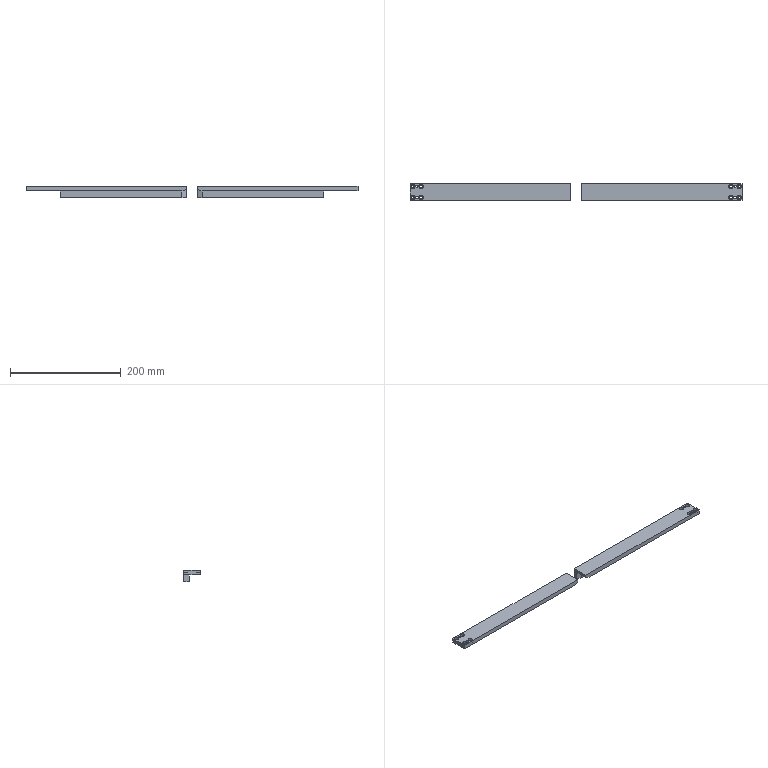Part | 2 solids | 56 faces | box 600 x 30 x 20 mm | volume 190506 mm3 | plane 34 | cylinder 22 | commonest cylinder face diameters 4.5 x8 8 x8 4 x6
STEP:
#1=CARTESIAN_POINT('',(145.,15.,-20.));
#2=VERTEX_POINT('',#1);
#3=CARTESIAN_POINT('',(145.,8.,-20.));
#4=VERTEX_POINT('',#3);
#5=CARTESIAN_POINT('',(145.,15.,-20.));
#6=DIRECTION('',(0.,-1.,0.));
#7=VECTOR('',#6,1000.);
#8=LINE('',#5,#7);
#9=EDGE_CURVE('',#2,#4,#8,.T.);
#10=ORIENTED_EDGE('',*,*,#9,.T.);
#11=CARTESIAN_POINT('',(136.758,5.,-20.));
#12=VERTEX_POINT('',#11);
#13=CARTESIAN_POINT('',(136.758,5.,-20.));
#14=DIRECTION('',(-0.9397,-0.342,0.));
#15=VECTOR('',#14,1000.);
#16=LINE('',#13,#15);
#17=EDGE_CURVE('',#4,#12,#16,.T.);
#18=ORIENTED_EDGE('',*,*,#17,.T.);
#19=CARTESIAN_POINT('',(-83.5,5.,-20.));
#20=VERTEX_POINT('',#19);
#21=CARTESIAN_POINT('',(-145.,5.,-20.));
#22=DIRECTION('',(1.,0.,0.));
#23=VECTOR('',#22,1000.);
#24=LINE('',#21,#23);
#25=EDGE_CURVE('',#20,#12,#24,.T.);
#26=ORIENTED_EDGE('',*,*,#25,.F.);
#27=CARTESIAN_POINT('',(-83.5,15.,-20.));
#28=VERTEX_POINT('',#27);
#29=CARTESIAN_POINT('',(-83.5,5.,-20.));
#30=DIRECTION('',(0.,1.,0.));
#31=VECTOR('',#30,1000.);
#32=LINE('',#29,#31);
#33=EDGE_CURVE('',#20,#28,#32,.T.);
#34=ORIENTED_EDGE('',*,*,#33,.T.);
#35=CARTESIAN_POINT('',(145.,15.,-20.));
#36=DIRECTION('',(-1.,0.,0.));
#37=VECTOR('',#36,1000.);
#38=LINE('',#35,#37);
#39=EDGE_CURVE('',#2,#28,#38,.T.);
#40=ORIENTED_EDGE('',*,*,#39,.F.);
#41=EDGE_LOOP('',(#10,#18,#26,#34,#40));
#42=FACE_BOUND('',#41,.T.);
#43=CARTESIAN_POINT('',(145.,15.,-20.));
#44=DIRECTION('',(0.,0.,1.));
#45=DIRECTION('',(-1.,0.,0.));
#46=AXIS2_PLACEMENT_3D('',#43,#44,#45);
#47=PLANE('',#46);
#48=ADVANCED_FACE('',(#42),#47,.F.);
#49=CARTESIAN_POINT('',(-145.,15.,-8.));
#50=VERTEX_POINT('',#49);
#51=CARTESIAN_POINT('',(-145.,15.,0.));
#52=VERTEX_POINT('',#51);
#53=CARTESIAN_POINT('',(-145.,15.,-20.));
#54=DIRECTION('',(0.,0.,1.));
#55=VECTOR('',#54,1000.);
#56=LINE('',#53,#55);
#57=EDGE_CURVE('',#50,#52,#56,.T.);
#58=ORIENTED_EDGE('',*,*,#57,.F.);
#59=CARTESIAN_POINT('',(-145.,-15.,-8.));
#60=VERTEX_POINT('',#59);
#61=CARTESIAN_POINT('',(-145.,-15.,-8.));
#62=DIRECTION('',(0.,-1.,0.));
#63=VECTOR('',#62,1000.);
#64=LINE('',#61,#63);
#65=EDGE_CURVE('',#50,#60,#64,.T.);
#66=ORIENTED_EDGE('',*,*,#65,.T.);
#67=CARTESIAN_POINT('',(-145.,-15.,0.));
#68=VERTEX_POINT('',#67);
#69=CARTESIAN_POINT('',(-145.,-15.,-20.));
#70=DIRECTION('',(0.,0.,1.));
#71=VECTOR('',#70,1000.);
#72=LINE('',#69,#71);
#73=EDGE_CURVE('',#60,#68,#72,.T.);
#74=ORIENTED_EDGE('',*,*,#73,.T.);
#75=CARTESIAN_POINT('',(-145.,15.,0.));
#76=DIRECTION('',(0.,-1.,0.));
#77=VECTOR('',#76,1000.);
#78=LINE('',#75,#77);
#79=EDGE_CURVE('',#52,#68,#78,.T.);
#80=ORIENTED_EDGE('',*,*,#79,.F.);
#81=EDGE_LOOP('',(#58,#66,#74,#80));
#82=FACE_BOUND('',#81,.T.);
#83=CARTESIAN_POINT('',(-145.,15.,-20.));
#84=DIRECTION('',(1.,0.,0.));
#85=DIRECTION('',(0.,0.,1.));
#86=AXIS2_PLACEMENT_3D('',#83,#84,#85);
#87=PLANE('',#86);
#88=ADVANCED_FACE('',(#82),#87,.F.);
#89=CARTESIAN_POINT('',(-134.5,-9.5,0.));
#90=VERTEX_POINT('',#89);
#91=CARTESIAN_POINT('',(-134.5,-10.5,0.));
#92=VERTEX_POINT('',#91);
#93=CARTESIAN_POINT('',(-134.5,-9.5,0.));
#94=DIRECTION('',(0.,-1.,0.));
#95=VECTOR('',#94,1000.);
#96=LINE('',#93,#95);
#97=EDGE_CURVE('',#90,#92,#96,.T.);
#98=ORIENTED_EDGE('',*,*,#97,.F.);
#99=CARTESIAN_POINT('',(-130.5,-9.5,0.));
#100=VERTEX_POINT('',#99);
#101=CARTESIAN_POINT('',(-132.5,-9.5,0.));
#102=DIRECTION('',(0.,0.,1.));
#103=DIRECTION('',(1.,0.,0.));
#104=AXIS2_PLACEMENT_3D('',#101,#102,#103);
#105=CIRCLE('',#104,2.);
#106=EDGE_CURVE('',#100,#90,#105,.T.);
#107=ORIENTED_EDGE('',*,*,#106,.F.);
#108=CARTESIAN_POINT('',(-130.5,-10.5,0.));
#109=VERTEX_POINT('',#108);
#110=CARTESIAN_POINT('',(-130.5,-9.5,0.));
#111=DIRECTION('',(0.,1.,0.));
#112=VECTOR('',#111,1000.);
#113=LINE('',#110,#112);
#114=EDGE_CURVE('',#109,#100,#113,.T.);
#115=ORIENTED_EDGE('',*,*,#114,.F.);
#116=CARTESIAN_POINT('',(-132.5,-10.5,0.));
#117=DIRECTION('',(0.,0.,1.));
#118=DIRECTION('',(1.,0.,0.));
#119=AXIS2_PLACEMENT_3D('',#116,#117,#118);
#120=CIRCLE('',#119,2.);
#121=EDGE_CURVE('',#92,#109,#120,.T.);
#122=ORIENTED_EDGE('',*,*,#121,.F.);
#123=EDGE_LOOP('',(#98,#107,#115,#122));
#124=FACE_BOUND('',#123,.T.);
#125=CARTESIAN_POINT('',(-130.5,10.,0.));
#126=VERTEX_POINT('',#125);
#127=CARTESIAN_POINT('',(-132.5,10.,0.));
#128=DIRECTION('',(0.,0.,1.));
#129=DIRECTION('',(1.,0.,0.));
#130=AXIS2_PLACEMENT_3D('',#127,#128,#129);
#131=CIRCLE('',#130,2.);
#132=EDGE_CURVE('',#126,#126,#131,.T.);
#133=ORIENTED_EDGE('',*,*,#132,.F.);
#134=EDGE_LOOP('',(#133));
#135=FACE_BOUND('',#134,.T.);
#136=CARTESIAN_POINT('',(-136.,10.,0.));
#137=VERTEX_POINT('',#136);
#138=CARTESIAN_POINT('',(-140.,10.,0.));
#139=DIRECTION('',(0.,0.,1.));
#140=DIRECTION('',(1.,0.,0.));
#141=AXIS2_PLACEMENT_3D('',#138,#139,#140);
#142=CIRCLE('',#141,4.);
#143=EDGE_CURVE('',#137,#137,#142,.T.);
#144=ORIENTED_EDGE('',*,*,#143,.F.);
#145=EDGE_LOOP('',(#144));
#146=FACE_BOUND('',#145,.T.);
#147=CARTESIAN_POINT('',(-136.,-10.,0.));
#148=VERTEX_POINT('',#147);
#149=CARTESIAN_POINT('',(-140.,-10.,0.));
#150=DIRECTION('',(0.,0.,1.));
#151=DIRECTION('',(1.,0.,0.));
#152=AXIS2_PLACEMENT_3D('',#149,#150,#151);
#153=CIRCLE('',#152,4.);
#154=EDGE_CURVE('',#148,#148,#153,.T.);
#155=ORIENTED_EDGE('',*,*,#154,.F.);
#156=EDGE_LOOP('',(#155));
#157=FACE_BOUND('',#156,.T.);
#158=CARTESIAN_POINT('',(-121.,-10.,0.));
#159=VERTEX_POINT('',#158);
#160=CARTESIAN_POINT('',(-125.,-10.,0.));
#161=DIRECTION('',(0.,0.,1.));
#162=DIRECTION('',(1.,0.,0.));
#163=AXIS2_PLACEMENT_3D('',#160,#161,#162);
#164=CIRCLE('',#163,4.);
#165=EDGE_CURVE('',#159,#159,#164,.T.);
#166=ORIENTED_EDGE('',*,*,#165,.F.);
#167=EDGE_LOOP('',(#166));
#168=FACE_BOUND('',#167,.T.);
#169=CARTESIAN_POINT('',(-121.,10.,0.));
#170=VERTEX_POINT('',#169);
#171=CARTESIAN_POINT('',(-125.,10.,0.));
#172=DIRECTION('',(0.,0.,1.));
#173=DIRECTION('',(1.,0.,0.));
#174=AXIS2_PLACEMENT_3D('',#171,#172,#173);
#175=CIRCLE('',#174,4.);
#176=EDGE_CURVE('',#170,#170,#175,.T.);
#177=ORIENTED_EDGE('',*,*,#176,.F.);
#178=EDGE_LOOP('',(#177));
#179=FACE_BOUND('',#178,.T.);
#180=CARTESIAN_POINT('',(145.,-15.,0.));
#181=VERTEX_POINT('',#180);
#182=CARTESIAN_POINT('',(145.,-15.,0.));
#183=DIRECTION('',(1.,0.,0.));
#184=VECTOR('',#183,1000.);
#185=LINE('',#182,#184);
#186=EDGE_CURVE('',#68,#181,#185,.T.);
#187=ORIENTED_EDGE('',*,*,#186,.T.);
#188=CARTESIAN_POINT('',(145.,15.,0.));
#189=VERTEX_POINT('',#188);
#190=CARTESIAN_POINT('',(145.,15.,0.));
#191=DIRECTION('',(0.,-1.,0.));
#192=VECTOR('',#191,1000.);
#193=LINE('',#190,#192);
#194=EDGE_CURVE('',#189,#181,#193,.T.);
#195=ORIENTED_EDGE('',*,*,#194,.F.);
#196=CARTESIAN_POINT('',(145.,15.,0.));
#197=DIRECTION('',(1.,0.,0.));
#198=VECTOR('',#197,1000.);
#199=LINE('',#196,#198);
#200=EDGE_CURVE('',#52,#189,#199,.T.);
#201=ORIENTED_EDGE('',*,*,#200,.F.);
#202=ORIENTED_EDGE('',*,*,#79,.T.);
#203=EDGE_LOOP('',(#187,#195,#201,#202));
#204=FACE_BOUND('',#203,.T.);
#205=CARTESIAN_POINT('',(145.,15.,0.));
#206=DIRECTION('',(0.,0.,-1.));
#207=DIRECTION('',(1.,0.,0.));
#208=AXIS2_PLACEMENT_3D('',#205,#206,#207);
#209=PLANE('',#208);
#210=ADVANCED_FACE('',(#124,#135,#146,#157,#168,#179,#204),#209,.F.);
#211=CARTESIAN_POINT('',(145.,-15.,-5.));
#212=VERTEX_POINT('',#211);
#213=CARTESIAN_POINT('',(145.,8.,-5.));
#214=VERTEX_POINT('',#213);
#215=CARTESIAN_POINT('',(145.,15.,-5.));
#216=DIRECTION('',(0.,1.,0.));
#217=VECTOR('',#216,1000.);
#218=LINE('',#215,#217);
#219=EDGE_CURVE('',#212,#214,#218,.T.);
#220=ORIENTED_EDGE('',*,*,#219,.T.);
#221=CARTESIAN_POINT('',(145.,8.,-20.));
#222=DIRECTION('',(0.,0.,-1.));
#223=VECTOR('',#222,1000.);
#224=LINE('',#221,#223);
#225=EDGE_CURVE('',#214,#4,#224,.T.);
#226=ORIENTED_EDGE('',*,*,#225,.T.);
#227=ORIENTED_EDGE('',*,*,#9,.F.);
#228=CARTESIAN_POINT('',(145.,15.,-20.));
#229=DIRECTION('',(0.,0.,-1.));
#230=VECTOR('',#229,1000.);
#231=LINE('',#228,#230);
#232=EDGE_CURVE('',#189,#2,#231,.T.);
#233=ORIENTED_EDGE('',*,*,#232,.F.);
#234=ORIENTED_EDGE('',*,*,#194,.T.);
#235=CARTESIAN_POINT('',(145.,-15.,-20.));
#236=DIRECTION('',(0.,0.,-1.));
#237=VECTOR('',#236,1000.);
#238=LINE('',#235,#237);
#239=EDGE_CURVE('',#181,#212,#238,.T.);
#240=ORIENTED_EDGE('',*,*,#239,.T.);
#241=EDGE_LOOP('',(#220,#226,#227,#233,#234,#240));
#242=FACE_BOUND('',#241,.T.);
#243=CARTESIAN_POINT('',(145.,15.,-20.));
#244=DIRECTION('',(-1.,0.,0.));
#245=DIRECTION('',(0.,0.,-1.));
#246=AXIS2_PLACEMENT_3D('',#243,#244,#245);
#247=PLANE('',#246);
#248=ADVANCED_FACE('',(#242),#247,.F.);
#249=CARTESIAN_POINT('',(-83.5,15.,-8.));
#250=VERTEX_POINT('',#249);
#251=CARTESIAN_POINT('',(-83.5,15.,-20.));
#252=DIRECTION('',(0.,0.,-1.));
#253=VECTOR('',#252,1000.);
#254=LINE('',#251,#253);
#255=EDGE_CURVE('',#250,#28,#254,.T.);
#256=ORIENTED_EDGE('',*,*,#255,.F.);
#257=CARTESIAN_POINT('',(-145.,15.,-8.));
#258=DIRECTION('',(1.,0.,0.));
#259=VECTOR('',#258,1000.);
#260=LINE('',#257,#259);
#261=EDGE_CURVE('',#50,#250,#260,.T.);
#262=ORIENTED_EDGE('',*,*,#261,.F.);
#263=ORIENTED_EDGE('',*,*,#57,.T.);
#264=ORIENTED_EDGE('',*,*,#200,.T.);
#265=ORIENTED_EDGE('',*,*,#232,.T.);
#266=ORIENTED_EDGE('',*,*,#39,.T.);
#267=EDGE_LOOP('',(#256,#262,#263,#264,#265,#266));
#268=FACE_BOUND('',#267,.T.);
#269=CARTESIAN_POINT('',(-145.,15.,-20.));
#270=DIRECTION('',(0.,1.,0.));
#271=DIRECTION('',(1.,0.,0.));
#272=AXIS2_PLACEMENT_3D('',#269,#270,#271);
#273=PLANE('',#272);
#274=ADVANCED_FACE('',(#268),#273,.T.);
#275=CARTESIAN_POINT('',(136.758,-15.,-8.));
#276=VERTEX_POINT('',#275);
#277=CARTESIAN_POINT('',(-145.,-15.,-8.));
#278=DIRECTION('',(1.,0.,0.));
#279=VECTOR('',#278,1000.);
#280=LINE('',#277,#279);
#281=EDGE_CURVE('',#60,#276,#280,.T.);
#282=ORIENTED_EDGE('',*,*,#281,.T.);
#283=CARTESIAN_POINT('',(136.758,-15.,-8.));
#284=DIRECTION('',(0.9397,0.,0.342));
#285=VECTOR('',#284,1000.);
#286=LINE('',#283,#285);
#287=EDGE_CURVE('',#276,#212,#286,.T.);
#288=ORIENTED_EDGE('',*,*,#287,.T.);
#289=ORIENTED_EDGE('',*,*,#239,.F.);
#290=ORIENTED_EDGE('',*,*,#186,.F.);
#291=ORIENTED_EDGE('',*,*,#73,.F.);
#292=EDGE_LOOP('',(#282,#288,#289,#290,#291));
#293=FACE_BOUND('',#292,.T.);
#294=CARTESIAN_POINT('',(-145.,-15.,-20.));
#295=DIRECTION('',(0.,1.,0.));
#296=DIRECTION('',(1.,0.,0.));
#297=AXIS2_PLACEMENT_3D('',#294,#295,#296);
#298=PLANE('',#297);
#299=ADVANCED_FACE('',(#293),#298,.F.);
#300=CARTESIAN_POINT('',(-130.5,-10.5,-8.));
#301=VERTEX_POINT('',#300);
#302=CARTESIAN_POINT('',(-130.5,-9.5,-8.));
#303=VERTEX_POINT('',#302);
#304=CARTESIAN_POINT('',(-130.5,-15.,-8.));
#305=DIRECTION('',(0.,1.,0.));
#306=VECTOR('',#305,1000.);
#307=LINE('',#304,#306);
#308=EDGE_CURVE('',#301,#303,#307,.T.);
#309=ORIENTED_EDGE('',*,*,#308,.T.);
#310=CARTESIAN_POINT('',(-134.5,-9.5,-8.));
#311=VERTEX_POINT('',#310);
#312=CARTESIAN_POINT('',(-132.5,-9.5,-8.));
#313=DIRECTION('',(0.,0.,1.));
#314=DIRECTION('',(1.,0.,0.));
#315=AXIS2_PLACEMENT_3D('',#312,#313,#314);
#316=CIRCLE('',#315,2.);
#317=EDGE_CURVE('',#303,#311,#316,.T.);
#318=ORIENTED_EDGE('',*,*,#317,.T.);
#319=CARTESIAN_POINT('',(-134.5,-10.5,-8.));
#320=VERTEX_POINT('',#319);
#321=CARTESIAN_POINT('',(-134.5,-15.,-8.));
#322=DIRECTION('',(0.,-1.,0.));
#323=VECTOR('',#322,1000.);
#324=LINE('',#321,#323);
#325=EDGE_CURVE('',#311,#320,#324,.T.);
#326=ORIENTED_EDGE('',*,*,#325,.T.);
#327=CARTESIAN_POINT('',(-132.5,-10.5,-8.));
#328=DIRECTION('',(0.,0.,1.));
#329=DIRECTION('',(1.,0.,0.));
#330=AXIS2_PLACEMENT_3D('',#327,#328,#329);
#331=CIRCLE('',#330,2.);
#332=EDGE_CURVE('',#320,#301,#331,.T.);
#333=ORIENTED_EDGE('',*,*,#332,.T.);
#334=EDGE_LOOP('',(#309,#318,#326,#333));
#335=FACE_BOUND('',#334,.T.);
#336=CARTESIAN_POINT('',(-130.5,10.,-8.));
#337=VERTEX_POINT('',#336);
#338=CARTESIAN_POINT('',(-132.5,10.,-8.));
#339=DIRECTION('',(0.,0.,1.));
#340=DIRECTION('',(1.,0.,0.));
#341=AXIS2_PLACEMENT_3D('',#338,#339,#340);
#342=CIRCLE('',#341,2.);
#343=EDGE_CURVE('',#337,#337,#342,.T.);
#344=ORIENTED_EDGE('',*,*,#343,.T.);
#345=EDGE_LOOP('',(#344));
#346=FACE_BOUND('',#345,.T.);
#347=CARTESIAN_POINT('',(-137.75,10.,-8.));
#348=VERTEX_POINT('',#347);
#349=CARTESIAN_POINT('',(-140.,10.,-8.));
#350=DIRECTION('',(0.,0.,1.));
#351=DIRECTION('',(1.,0.,0.));
#352=AXIS2_PLACEMENT_3D('',#349,#350,#351);
#353=CIRCLE('',#352,2.25);
#354=EDGE_CURVE('',#348,#348,#353,.T.);
#355=ORIENTED_EDGE('',*,*,#354,.T.);
#356=EDGE_LOOP('',(#355));
#357=FACE_BOUND('',#356,.T.);
#358=CARTESIAN_POINT('',(-137.75,-10.,-8.));
#359=VERTEX_POINT('',#358);
#360=CARTESIAN_POINT('',(-140.,-10.,-8.));
#361=DIRECTION('',(0.,0.,1.));
#362=DIRECTION('',(1.,0.,0.));
#363=AXIS2_PLACEMENT_3D('',#360,#361,#362);
#364=CIRCLE('',#363,2.25);
#365=EDGE_CURVE('',#359,#359,#364,.T.);
#366=ORIENTED_EDGE('',*,*,#365,.T.);
#367=EDGE_LOOP('',(#366));
#368=FACE_BOUND('',#367,.T.);
#369=CARTESIAN_POINT('',(-122.75,-10.,-8.));
#370=VERTEX_POINT('',#369);
#371=CARTESIAN_POINT('',(-125.,-10.,-8.));
#372=DIRECTION('',(0.,0.,1.));
#373=DIRECTION('',(1.,0.,0.));
#374=AXIS2_PLACEMENT_3D('',#371,#372,#373);
#375=CIRCLE('',#374,2.25);
#376=EDGE_CURVE('',#370,#370,#375,.T.);
#377=ORIENTED_EDGE('',*,*,#376,.T.);
#378=EDGE_LOOP('',(#377));
#379=FACE_BOUND('',#378,.T.);
#380=CARTESIAN_POINT('',(-122.75,10.,-8.));
#381=VERTEX_POINT('',#380);
#382=CARTESIAN_POINT('',(-125.,10.,-8.));
#383=DIRECTION('',(0.,0.,1.));
#384=DIRECTION('',(1.,0.,0.));
#385=AXIS2_PLACEMENT_3D('',#382,#383,#384);
#386=CIRCLE('',#385,2.25);
#387=EDGE_CURVE('',#381,#381,#386,.T.);
#388=ORIENTED_EDGE('',*,*,#387,.T.);
#389=EDGE_LOOP('',(#388));
#390=FACE_BOUND('',#389,.T.);
#391=CARTESIAN_POINT('',(-83.5,5.,-8.));
#392=VERTEX_POINT('',#391);
#393=CARTESIAN_POINT('',(136.758,5.,-8.));
#394=VERTEX_POINT('',#393);
#395=CARTESIAN_POINT('',(-145.,5.,-8.));
#396=DIRECTION('',(1.,0.,0.));
#397=VECTOR('',#396,1000.);
#398=LINE('',#395,#397);
#399=EDGE_CURVE('',#392,#394,#398,.T.);
#400=ORIENTED_EDGE('',*,*,#399,.T.);
#401=CARTESIAN_POINT('',(136.758,-15.,-8.));
#402=DIRECTION('',(0.,-1.,0.));
#403=VECTOR('',#402,1000.);
#404=LINE('',#401,#403);
#405=EDGE_CURVE('',#394,#276,#404,.T.);
#406=ORIENTED_EDGE('',*,*,#405,.T.);
#407=ORIENTED_EDGE('',*,*,#281,.F.);
#408=ORIENTED_EDGE('',*,*,#65,.F.);
#409=ORIENTED_EDGE('',*,*,#261,.T.);
#410=CARTESIAN_POINT('',(-83.5,5.,-8.));
#411=DIRECTION('',(0.,1.,0.));
#412=VECTOR('',#411,1000.);
#413=LINE('',#410,#412);
#414=EDGE_CURVE('',#392,#250,#413,.T.);
#415=ORIENTED_EDGE('',*,*,#414,.F.);
#416=EDGE_LOOP('',(#400,#406,#407,#408,#409,#415));
#417=FACE_BOUND('',#416,.T.);
#418=CARTESIAN_POINT('',(-145.,-15.,-8.));
#419=DIRECTION('',(0.,0.,1.));
#420=DIRECTION('',(-1.,0.,0.));
#421=AXIS2_PLACEMENT_3D('',#418,#419,#420);
#422=PLANE('',#421);
#423=ADVANCED_FACE('',(#335,#346,#357,#368,#379,#390,#417),#422,.F.);
#424=ORIENTED_EDGE('',*,*,#25,.T.);
#425=CARTESIAN_POINT('',(136.758,5.,-20.));
#426=DIRECTION('',(0.,0.,1.));
#427=VECTOR('',#426,1000.);
#428=LINE('',#425,#427);
#429=EDGE_CURVE('',#12,#394,#428,.T.);
#430=ORIENTED_EDGE('',*,*,#429,.T.);
#431=ORIENTED_EDGE('',*,*,#399,.F.);
#432=CARTESIAN_POINT('',(-83.5,5.,-20.));
#433=DIRECTION('',(0.,0.,-1.));
#434=VECTOR('',#433,1000.);
#435=LINE('',#432,#434);
#436=EDGE_CURVE('',#392,#20,#435,.T.);
#437=ORIENTED_EDGE('',*,*,#436,.T.);
#438=EDGE_LOOP('',(#424,#430,#431,#437));
#439=FACE_BOUND('',#438,.T.);
#440=CARTESIAN_POINT('',(-145.,5.,-20.));
#441=DIRECTION('',(0.,1.,0.));
#442=DIRECTION('',(0.,0.,1.));
#443=AXIS2_PLACEMENT_3D('',#440,#441,#442);
#444=PLANE('',#443);
#445=ADVANCED_FACE('',(#439),#444,.F.);
#446=ORIENTED_EDGE('',*,*,#255,.T.);
#447=ORIENTED_EDGE('',*,*,#33,.F.);
#448=ORIENTED_EDGE('',*,*,#436,.F.);
#449=ORIENTED_EDGE('',*,*,#414,.T.);
#450=EDGE_LOOP('',(#446,#447,#448,#449));
#451=FACE_BOUND('',#450,.T.);
#452=CARTESIAN_POINT('',(-83.5,5.,-20.));
#453=DIRECTION('',(1.,0.,0.));
#454=DIRECTION('',(0.,0.,1.));
#455=AXIS2_PLACEMENT_3D('',#452,#453,#454);
#456=PLANE('',#455);
#457=ADVANCED_FACE('',(#451),#456,.F.);
#458=CARTESIAN_POINT('',(-122.75,10.,-4.4));
#459=VERTEX_POINT('',#458);
#460=CARTESIAN_POINT('',(-125.,10.,-4.4));
#461=DIRECTION('',(0.,0.,1.));
#462=DIRECTION('',(1.,0.,0.));
#463=AXIS2_PLACEMENT_3D('',#460,#461,#462);
#464=CIRCLE('',#463,2.25);
#465=EDGE_CURVE('',#459,#459,#464,.T.);
#466=ORIENTED_EDGE('',*,*,#465,.T.);
#467=EDGE_LOOP('',(#466));
#468=FACE_BOUND('',#467,.T.);
#469=ORIENTED_EDGE('',*,*,#387,.F.);
#470=EDGE_LOOP('',(#469));
#471=FACE_BOUND('',#470,.T.);
#472=CARTESIAN_POINT('',(-125.,10.,0.));
#473=DIRECTION('',(0.,0.,1.));
#474=DIRECTION('',(-1.,0.,0.));
#475=AXIS2_PLACEMENT_3D('',#472,#473,#474);
#476=CYLINDRICAL_SURFACE('',#475,2.25);
#477=ADVANCED_FACE('',(#468,#471),#476,.F.);
#478=ORIENTED_EDGE('',*,*,#465,.F.);
#479=EDGE_LOOP('',(#478));
#480=FACE_BOUND('',#479,.T.);
#481=CARTESIAN_POINT('',(-121.,10.,-4.4));
#482=VERTEX_POINT('',#481);
#483=CARTESIAN_POINT('',(-125.,10.,-4.4));
#484=DIRECTION('',(0.,0.,1.));
#485=DIRECTION('',(1.,0.,0.));
#486=AXIS2_PLACEMENT_3D('',#483,#484,#485);
#487=CIRCLE('',#486,4.);
#488=EDGE_CURVE('',#482,#482,#487,.T.);
#489=ORIENTED_EDGE('',*,*,#488,.T.);
#490=EDGE_LOOP('',(#489));
#491=FACE_BOUND('',#490,.T.);
#492=CARTESIAN_POINT('',(-125.,12.25,-4.4));
#493=DIRECTION('',(0.,0.,-1.));
#494=DIRECTION('',(1.,0.,0.));
#495=AXIS2_PLACEMENT_3D('',#492,#493,#494);
#496=PLANE('',#495);
#497=ADVANCED_FACE('',(#480,#491),#496,.F.);
#498=ORIENTED_EDGE('',*,*,#488,.F.);
#499=EDGE_LOOP('',(#498));
#500=FACE_BOUND('',#499,.T.);
#501=ORIENTED_EDGE('',*,*,#176,.T.);
#502=EDGE_LOOP('',(#501));
#503=FACE_BOUND('',#502,.T.);
#504=CARTESIAN_POINT('',(-125.,10.,0.));
#505=DIRECTION('',(0.,0.,1.));
#506=DIRECTION('',(-1.,0.,0.));
#507=AXIS2_PLACEMENT_3D('',#504,#505,#506);
#508=CYLINDRICAL_SURFACE('',#507,4.);
#509=ADVANCED_FACE('',(#500,#503),#508,.F.);
#510=CARTESIAN_POINT('',(-122.75,-10.,-4.4));
#511=VERTEX_POINT('',#510);
#512=CARTESIAN_POINT('',(-125.,-10.,-4.4));
#513=DIRECTION('',(0.,0.,1.));
#514=DIRECTION('',(1.,0.,0.));
#515=AXIS2_PLACEMENT_3D('',#512,#513,#514);
#516=CIRCLE('',#515,2.25);
#517=EDGE_CURVE('',#511,#511,#516,.T.);
#518=ORIENTED_EDGE('',*,*,#517,.T.);
#519=EDGE_LOOP('',(#518));
#520=FACE_BOUND('',#519,.T.);
#521=ORIENTED_EDGE('',*,*,#376,.F.);
#522=EDGE_LOOP('',(#521));
#523=FACE_BOUND('',#522,.T.);
#524=CARTESIAN_POINT('',(-125.,-10.,0.));
#525=DIRECTION('',(0.,0.,1.));
#526=DIRECTION('',(-1.,0.,0.));
#527=AXIS2_PLACEMENT_3D('',#524,#525,#526);
#528=CYLINDRICAL_SURFACE('',#527,2.25);
#529=ADVANCED_FACE('',(#520,#523),#528,.F.);
#530=ORIENTED_EDGE('',*,*,#517,.F.);
#531=EDGE_LOOP('',(#530));
#532=FACE_BOUND('',#531,.T.);
#533=CARTESIAN_POINT('',(-121.,-10.,-4.4));
#534=VERTEX_POINT('',#533);
#535=CARTESIAN_POINT('',(-125.,-10.,-4.4));
#536=DIRECTION('',(0.,0.,1.));
#537=DIRECTION('',(1.,0.,0.));
#538=AXIS2_PLACEMENT_3D('',#535,#536,#537);
#539=CIRCLE('',#538,4.);
#540=EDGE_CURVE('',#534,#534,#539,.T.);
#541=ORIENTED_EDGE('',*,*,#540,.T.);
#542=EDGE_LOOP('',(#541));
#543=FACE_BOUND('',#542,.T.);
#544=CARTESIAN_POINT('',(-125.,-7.75,-4.4));
#545=DIRECTION('',(0.,0.,-1.));
#546=DIRECTION('',(1.,0.,0.));
#547=AXIS2_PLACEMENT_3D('',#544,#545,#546);
#548=PLANE('',#547);
#549=ADVANCED_FACE('',(#532,#543),#548,.F.);
#550=ORIENTED_EDGE('',*,*,#540,.F.);
#551=EDGE_LOOP('',(#550));
#552=FACE_BOUND('',#551,.T.);
#553=ORIENTED_EDGE('',*,*,#165,.T.);
#554=EDGE_LOOP('',(#553));
#555=FACE_BOUND('',#554,.T.);
#556=CARTESIAN_POINT('',(-125.,-10.,0.));
#557=DIRECTION('',(0.,0.,1.));
#558=DIRECTION('',(-1.,0.,0.));
#559=AXIS2_PLACEMENT_3D('',#556,#557,#558);
#560=CYLINDRICAL_SURFACE('',#559,4.);
#561=ADVANCED_FACE('',(#552,#555),#560,.F.);
#562=CARTESIAN_POINT('',(-137.75,-10.,-4.4));
#563=VERTEX_POINT('',#562);
#564=CARTESIAN_POINT('',(-140.,-10.,-4.4));
#565=DIRECTION('',(0.,0.,1.));
#566=DIRECTION('',(1.,0.,0.));
#567=AXIS2_PLACEMENT_3D('',#564,#565,#566);
#568=CIRCLE('',#567,2.25);
#569=EDGE_CURVE('',#563,#563,#568,.T.);
#570=ORIENTED_EDGE('',*,*,#569,.T.);
#571=EDGE_LOOP('',(#570));
#572=FACE_BOUND('',#571,.T.);
#573=ORIENTED_EDGE('',*,*,#365,.F.);
#574=EDGE_LOOP('',(#573));
#575=FACE_BOUND('',#574,.T.);
#576=CARTESIAN_POINT('',(-140.,-10.,0.));
#577=DIRECTION('',(0.,0.,1.));
#578=DIRECTION('',(-1.,0.,0.));
#579=AXIS2_PLACEMENT_3D('',#576,#577,#578);
#580=CYLINDRICAL_SURFACE('',#579,2.25);
#581=ADVANCED_FACE('',(#572,#575),#580,.F.);
#582=ORIENTED_EDGE('',*,*,#569,.F.);
#583=EDGE_LOOP('',(#582));
#584=FACE_BOUND('',#583,.T.);
#585=CARTESIAN_POINT('',(-136.,-10.,-4.4));
#586=VERTEX_POINT('',#585);
#587=CARTESIAN_POINT('',(-140.,-10.,-4.4));
#588=DIRECTION('',(0.,0.,1.));
#589=DIRECTION('',(1.,0.,0.));
#590=AXIS2_PLACEMENT_3D('',#587,#588,#589);
#591=CIRCLE('',#590,4.);
#592=EDGE_CURVE('',#586,#586,#591,.T.);
#593=ORIENTED_EDGE('',*,*,#592,.T.);
#594=EDGE_LOOP('',(#593));
#595=FACE_BOUND('',#594,.T.);
#596=CARTESIAN_POINT('',(-140.,-7.75,-4.4));
#597=DIRECTION('',(0.,0.,-1.));
#598=DIRECTION('',(1.,0.,0.));
#599=AXIS2_PLACEMENT_3D('',#596,#597,#598);
#600=PLANE('',#599);
#601=ADVANCED_FACE('',(#584,#595),#600,.F.);
#602=ORIENTED_EDGE('',*,*,#592,.F.);
#603=EDGE_LOOP('',(#602));
#604=FACE_BOUND('',#603,.T.);
#605=ORIENTED_EDGE('',*,*,#154,.T.);
#606=EDGE_LOOP('',(#605));
#607=FACE_BOUND('',#606,.T.);
#608=CARTESIAN_POINT('',(-140.,-10.,0.));
#609=DIRECTION('',(0.,0.,1.));
#610=DIRECTION('',(-1.,0.,0.));
#611=AXIS2_PLACEMENT_3D('',#608,#609,#610);
#612=CYLINDRICAL_SURFACE('',#611,4.);
#613=ADVANCED_FACE('',(#604,#607),#612,.F.);
#614=CARTESIAN_POINT('',(-137.75,10.,-4.4));
#615=VERTEX_POINT('',#614);
#616=CARTESIAN_POINT('',(-140.,10.,-4.4));
#617=DIRECTION('',(0.,0.,1.));
#618=DIRECTION('',(1.,0.,0.));
#619=AXIS2_PLACEMENT_3D('',#616,#617,#618);
#620=CIRCLE('',#619,2.25);
#621=EDGE_CURVE('',#615,#615,#620,.T.);
#622=ORIENTED_EDGE('',*,*,#621,.T.);
#623=EDGE_LOOP('',(#622));
#624=FACE_BOUND('',#623,.T.);
#625=ORIENTED_EDGE('',*,*,#354,.F.);
#626=EDGE_LOOP('',(#625));
#627=FACE_BOUND('',#626,.T.);
#628=CARTESIAN_POINT('',(-140.,10.,0.));
#629=DIRECTION('',(0.,0.,1.));
#630=DIRECTION('',(-1.,0.,0.));
#631=AXIS2_PLACEMENT_3D('',#628,#629,#630);
#632=CYLINDRICAL_SURFACE('',#631,2.25);
#633=ADVANCED_FACE('',(#624,#627),#632,.F.);
#634=ORIENTED_EDGE('',*,*,#621,.F.);
#635=EDGE_LOOP('',(#634));
#636=FACE_BOUND('',#635,.T.);
#637=CARTESIAN_POINT('',(-136.,10.,-4.4));
#638=VERTEX_POINT('',#637);
#639=CARTESIAN_POINT('',(-140.,10.,-4.4));
#640=DIRECTION('',(0.,0.,1.));
#641=DIRECTION('',(1.,0.,0.));
#642=AXIS2_PLACEMENT_3D('',#639,#640,#641);
#643=CIRCLE('',#642,4.);
#644=EDGE_CURVE('',#638,#638,#643,.T.);
#645=ORIENTED_EDGE('',*,*,#644,.T.);
#646=EDGE_LOOP('',(#645));
#647=FACE_BOUND('',#646,.T.);
#648=CARTESIAN_POINT('',(-140.,12.25,-4.4));
#649=DIRECTION('',(0.,0.,-1.));
#650=DIRECTION('',(1.,0.,0.));
#651=AXIS2_PLACEMENT_3D('',#648,#649,#650);
#652=PLANE('',#651);
#653=ADVANCED_FACE('',(#636,#647),#652,.F.);
#654=ORIENTED_EDGE('',*,*,#644,.F.);
#655=EDGE_LOOP('',(#654));
#656=FACE_BOUND('',#655,.T.);
#657=ORIENTED_EDGE('',*,*,#143,.T.);
#658=EDGE_LOOP('',(#657));
#659=FACE_BOUND('',#658,.T.);
#660=CARTESIAN_POINT('',(-140.,10.,0.));
#661=DIRECTION('',(0.,0.,1.));
#662=DIRECTION('',(-1.,0.,0.));
#663=AXIS2_PLACEMENT_3D('',#660,#661,#662);
#664=CYLINDRICAL_SURFACE('',#663,4.);
#665=ADVANCED_FACE('',(#656,#659),#664,.F.);
#666=ORIENTED_EDGE('',*,*,#287,.F.);
#667=ORIENTED_EDGE('',*,*,#405,.F.);
#668=CARTESIAN_POINT('',(133.305,3.743,-9.257));
#669=DIRECTION('',(-0.8891,-0.3236,-0.3236));
#670=VECTOR('',#669,1000.);
#671=LINE('',#668,#670);
#672=EDGE_CURVE('',#214,#394,#671,.T.);
#673=ORIENTED_EDGE('',*,*,#672,.F.);
#674=ORIENTED_EDGE('',*,*,#219,.F.);
#675=EDGE_LOOP('',(#666,#667,#673,#674));
#676=FACE_BOUND('',#675,.T.);
#677=CARTESIAN_POINT('',(136.758,-15.,-8.));
#678=DIRECTION('',(-0.342,0.,0.9397));
#679=DIRECTION('',(0.,1.,0.));
#680=AXIS2_PLACEMENT_3D('',#677,#678,#679);
#681=PLANE('',#680);
#682=ADVANCED_FACE('',(#676),#681,.F.);
#683=ORIENTED_EDGE('',*,*,#17,.F.);
#684=ORIENTED_EDGE('',*,*,#225,.F.);
#685=ORIENTED_EDGE('',*,*,#672,.T.);
#686=ORIENTED_EDGE('',*,*,#429,.F.);
#687=EDGE_LOOP('',(#683,#684,#685,#686));
#688=FACE_BOUND('',#687,.T.);
#689=CARTESIAN_POINT('',(136.758,5.,-20.));
#690=DIRECTION('',(-0.342,0.9397,0.));
#691=DIRECTION('',(0.,0.,-1.));
#692=AXIS2_PLACEMENT_3D('',#689,#690,#691);
#693=PLANE('',#692);
#694=ADVANCED_FACE('',(#688),#693,.F.);
#695=ORIENTED_EDGE('',*,*,#132,.T.);
#696=EDGE_LOOP('',(#695));
#697=FACE_BOUND('',#696,.T.);
#698=ORIENTED_EDGE('',*,*,#343,.F.);
#699=EDGE_LOOP('',(#698));
#700=FACE_BOUND('',#699,.T.);
#701=CARTESIAN_POINT('',(-132.5,10.,-20.));
#702=DIRECTION('',(0.,0.,1.));
#703=DIRECTION('',(-1.,0.,0.));
#704=AXIS2_PLACEMENT_3D('',#701,#702,#703);
#705=CYLINDRICAL_SURFACE('',#704,2.);
#706=ADVANCED_FACE('',(#697,#700),#705,.F.);
#707=CARTESIAN_POINT('',(-130.5,-9.5,-20.));
#708=DIRECTION('',(0.,0.,1.));
#709=VECTOR('',#708,1000.);
#710=LINE('',#707,#709);
#711=EDGE_CURVE('',#303,#100,#710,.T.);
#712=ORIENTED_EDGE('',*,*,#711,.T.);
#713=ORIENTED_EDGE('',*,*,#106,.T.);
#714=CARTESIAN_POINT('',(-134.5,-9.5,-20.));
#715=DIRECTION('',(0.,0.,1.));
#716=VECTOR('',#715,1000.);
#717=LINE('',#714,#716);
#718=EDGE_CURVE('',#311,#90,#717,.T.);
#719=ORIENTED_EDGE('',*,*,#718,.F.);
#720=ORIENTED_EDGE('',*,*,#317,.F.);
#721=EDGE_LOOP('',(#712,#713,#719,#720));
#722=FACE_BOUND('',#721,.T.);
#723=CARTESIAN_POINT('',(-132.5,-9.5,-20.));
#724=DIRECTION('',(0.,0.,1.));
#725=DIRECTION('',(-1.,0.,0.));
#726=AXIS2_PLACEMENT_3D('',#723,#724,#725);
#727=CYLINDRICAL_SURFACE('',#726,2.);
#728=ADVANCED_FACE('',(#722),#727,.F.);
#729=CARTESIAN_POINT('',(-130.5,-10.5,-20.));
#730=DIRECTION('',(0.,0.,1.));
#731=VECTOR('',#730,1000.);
#732=LINE('',#729,#731);
#733=EDGE_CURVE('',#301,#109,#732,.T.);
#734=ORIENTED_EDGE('',*,*,#733,.T.);
#735=ORIENTED_EDGE('',*,*,#114,.T.);
#736=ORIENTED_EDGE('',*,*,#711,.F.);
#737=ORIENTED_EDGE('',*,*,#308,.F.);
#738=EDGE_LOOP('',(#734,#735,#736,#737));
#739=FACE_BOUND('',#738,.T.);
#740=CARTESIAN_POINT('',(-130.5,-9.5,-20.));
#741=DIRECTION('',(1.,0.,0.));
#742=DIRECTION('',(0.,0.,1.));
#743=AXIS2_PLACEMENT_3D('',#740,#741,#742);
#744=PLANE('',#743);
#745=ADVANCED_FACE('',(#739),#744,.F.);
#746=CARTESIAN_POINT('',(-134.5,-10.5,-20.));
#747=DIRECTION('',(0.,0.,1.));
#748=VECTOR('',#747,1000.);
#749=LINE('',#746,#748);
#750=EDGE_CURVE('',#320,#92,#749,.T.);
#751=ORIENTED_EDGE('',*,*,#750,.T.);
#752=ORIENTED_EDGE('',*,*,#121,.T.);
#753=ORIENTED_EDGE('',*,*,#733,.F.);
#754=ORIENTED_EDGE('',*,*,#332,.F.);
#755=EDGE_LOOP('',(#751,#752,#753,#754));
#756=FACE_BOUND('',#755,.T.);
#757=CARTESIAN_POINT('',(-132.5,-10.5,-20.));
#758=DIRECTION('',(0.,0.,1.));
#759=DIRECTION('',(-1.,0.,0.));
#760=AXIS2_PLACEMENT_3D('',#757,#758,#759);
#761=CYLINDRICAL_SURFACE('',#760,2.);
#762=ADVANCED_FACE('',(#756),#761,.F.);
#763=ORIENTED_EDGE('',*,*,#718,.T.);
#764=ORIENTED_EDGE('',*,*,#97,.T.);
#765=ORIENTED_EDGE('',*,*,#750,.F.);
#766=ORIENTED_EDGE('',*,*,#325,.F.);
#767=EDGE_LOOP('',(#763,#764,#765,#766));
#768=FACE_BOUND('',#767,.T.);
#769=CARTESIAN_POINT('',(-134.5,-9.5,-20.));
#770=DIRECTION('',(-1.,0.,0.));
#771=DIRECTION('',(0.,0.,-1.));
#772=AXIS2_PLACEMENT_3D('',#769,#770,#771);
#773=PLANE('',#772);
#774=ADVANCED_FACE('',(#768),#773,.F.);
#775=CLOSED_SHELL('',(#48,#88,#210,#248,#274,#299,#423,#445,#457,#477,#497,#509,#529,#549,#561,#581,#601,#613,#633,#653,#665,#682,#694,#706,#728,#745,#762,#774));
#776=MANIFOLD_SOLID_BREP('',#775);
#777=CARTESIAN_POINT('',(165.,15.,-20.));
#778=VERTEX_POINT('',#777);
#779=CARTESIAN_POINT('',(165.,8.,-20.));
#780=VERTEX_POINT('',#779);
#781=CARTESIAN_POINT('',(165.,15.,-20.));
#782=DIRECTION('',(0.,-1.,0.));
#783=VECTOR('',#782,1000.);
#784=LINE('',#781,#783);
#785=EDGE_CURVE('',#778,#780,#784,.T.);
#786=ORIENTED_EDGE('',*,*,#785,.F.);
#787=CARTESIAN_POINT('',(393.5,15.,-20.));
#788=VERTEX_POINT('',#787);
#789=CARTESIAN_POINT('',(165.,15.,-20.));
#790=DIRECTION('',(1.,0.,0.));
#791=VECTOR('',#790,1000.);
#792=LINE('',#789,#791);
#793=EDGE_CURVE('',#778,#788,#792,.T.);
#794=ORIENTED_EDGE('',*,*,#793,.T.);
#795=CARTESIAN_POINT('',(393.5,5.,-20.));
#796=VERTEX_POINT('',#795);
#797=CARTESIAN_POINT('',(393.5,5.,-20.));
#798=DIRECTION('',(0.,1.,0.));
#799=VECTOR('',#798,1000.);
#800=LINE('',#797,#799);
#801=EDGE_CURVE('',#796,#788,#800,.T.);
#802=ORIENTED_EDGE('',*,*,#801,.F.);
#803=CARTESIAN_POINT('',(173.242,5.,-20.));
#804=VERTEX_POINT('',#803);
#805=CARTESIAN_POINT('',(455.,5.,-20.));
#806=DIRECTION('',(-1.,0.,0.));
#807=VECTOR('',#806,1000.);
#808=LINE('',#805,#807);
#809=EDGE_CURVE('',#796,#804,#808,.T.);
#810=ORIENTED_EDGE('',*,*,#809,.T.);
#811=CARTESIAN_POINT('',(173.242,5.,-20.));
#812=DIRECTION('',(0.9397,-0.342,0.));
#813=VECTOR('',#812,1000.);
#814=LINE('',#811,#813);
#815=EDGE_CURVE('',#780,#804,#814,.T.);
#816=ORIENTED_EDGE('',*,*,#815,.F.);
#817=EDGE_LOOP('',(#786,#794,#802,#810,#816));
#818=FACE_BOUND('',#817,.T.);
#819=CARTESIAN_POINT('',(165.,15.,-20.));
#820=DIRECTION('',(0.,0.,1.));
#821=DIRECTION('',(1.,0.,0.));
#822=AXIS2_PLACEMENT_3D('',#819,#820,#821);
#823=PLANE('',#822);
#824=ADVANCED_FACE('',(#818),#823,.F.);
#825=CARTESIAN_POINT('',(455.,15.,-8.));
#826=VERTEX_POINT('',#825);
#827=CARTESIAN_POINT('',(455.,15.,0.));
#828=VERTEX_POINT('',#827);
#829=CARTESIAN_POINT('',(455.,15.,-20.));
#830=DIRECTION('',(0.,0.,1.));
#831=VECTOR('',#830,1000.);
#832=LINE('',#829,#831);
#833=EDGE_CURVE('',#826,#828,#832,.T.);
#834=ORIENTED_EDGE('',*,*,#833,.T.);
#835=CARTESIAN_POINT('',(455.,-15.,0.));
#836=VERTEX_POINT('',#835);
#837=CARTESIAN_POINT('',(455.,15.,0.));
#838=DIRECTION('',(0.,-1.,0.));
#839=VECTOR('',#838,1000.);
#840=LINE('',#837,#839);
#841=EDGE_CURVE('',#828,#836,#840,.T.);
#842=ORIENTED_EDGE('',*,*,#841,.T.);
#843=CARTESIAN_POINT('',(455.,-15.,-8.));
#844=VERTEX_POINT('',#843);
#845=CARTESIAN_POINT('',(455.,-15.,-20.));
#846=DIRECTION('',(0.,0.,1.));
#847=VECTOR('',#846,1000.);
#848=LINE('',#845,#847);
#849=EDGE_CURVE('',#844,#836,#848,.T.);
#850=ORIENTED_EDGE('',*,*,#849,.F.);
#851=CARTESIAN_POINT('',(455.,-15.,-8.));
#852=DIRECTION('',(0.,-1.,0.));
#853=VECTOR('',#852,1000.);
#854=LINE('',#851,#853);
#855=EDGE_CURVE('',#826,#844,#854,.T.);
#856=ORIENTED_EDGE('',*,*,#855,.F.);
#857=EDGE_LOOP('',(#834,#842,#850,#856));
#858=FACE_BOUND('',#857,.T.);
#859=CARTESIAN_POINT('',(455.,15.,-20.));
#860=DIRECTION('',(-1.,0.,0.));
#861=DIRECTION('',(0.,0.,1.));
#862=AXIS2_PLACEMENT_3D('',#859,#860,#861);
#863=PLANE('',#862);
#864=ADVANCED_FACE('',(#858),#863,.F.);
#865=CARTESIAN_POINT('',(444.5,-9.5,0.));
#866=VERTEX_POINT('',#865);
#867=CARTESIAN_POINT('',(444.5,-10.5,0.));
#868=VERTEX_POINT('',#867);
#869=CARTESIAN_POINT('',(444.5,-9.5,0.));
#870=DIRECTION('',(0.,-1.,0.));
#871=VECTOR('',#870,1000.);
#872=LINE('',#869,#871);
#873=EDGE_CURVE('',#866,#868,#872,.T.);
#874=ORIENTED_EDGE('',*,*,#873,.T.);
#875=CARTESIAN_POINT('',(440.5,-10.5,0.));
#876=VERTEX_POINT('',#875);
#877=CARTESIAN_POINT('',(442.5,-10.5,0.));
#878=DIRECTION('',(0.,0.,-1.));
#879=DIRECTION('',(-1.,0.,0.));
#880=AXIS2_PLACEMENT_3D('',#877,#878,#879);
#881=CIRCLE('',#880,2.);
#882=EDGE_CURVE('',#868,#876,#881,.T.);
#883=ORIENTED_EDGE('',*,*,#882,.T.);
#884=CARTESIAN_POINT('',(440.5,-9.5,0.));
#885=VERTEX_POINT('',#884);
#886=CARTESIAN_POINT('',(440.5,-9.5,0.));
#887=DIRECTION('',(0.,1.,0.));
#888=VECTOR('',#887,1000.);
#889=LINE('',#886,#888);
#890=EDGE_CURVE('',#876,#885,#889,.T.);
#891=ORIENTED_EDGE('',*,*,#890,.T.);
#892=CARTESIAN_POINT('',(442.5,-9.5,0.));
#893=DIRECTION('',(0.,0.,-1.));
#894=DIRECTION('',(-1.,0.,0.));
#895=AXIS2_PLACEMENT_3D('',#892,#893,#894);
#896=CIRCLE('',#895,2.);
#897=EDGE_CURVE('',#885,#866,#896,.T.);
#898=ORIENTED_EDGE('',*,*,#897,.T.);
#899=EDGE_LOOP('',(#874,#883,#891,#898));
#900=FACE_BOUND('',#899,.T.);
#901=CARTESIAN_POINT('',(440.5,10.,0.));
#902=VERTEX_POINT('',#901);
#903=CARTESIAN_POINT('',(442.5,10.,0.));
#904=DIRECTION('',(0.,0.,-1.));
#905=DIRECTION('',(-1.,0.,0.));
#906=AXIS2_PLACEMENT_3D('',#903,#904,#905);
#907=CIRCLE('',#906,2.);
#908=EDGE_CURVE('',#902,#902,#907,.T.);
#909=ORIENTED_EDGE('',*,*,#908,.T.);
#910=EDGE_LOOP('',(#909));
#911=FACE_BOUND('',#910,.T.);
#912=CARTESIAN_POINT('',(446.,10.,0.));
#913=VERTEX_POINT('',#912);
#914=CARTESIAN_POINT('',(450.,10.,0.));
#915=DIRECTION('',(0.,0.,-1.));
#916=DIRECTION('',(-1.,0.,0.));
#917=AXIS2_PLACEMENT_3D('',#914,#915,#916);
#918=CIRCLE('',#917,4.);
#919=EDGE_CURVE('',#913,#913,#918,.T.);
#920=ORIENTED_EDGE('',*,*,#919,.T.);
#921=EDGE_LOOP('',(#920));
#922=FACE_BOUND('',#921,.T.);
#923=CARTESIAN_POINT('',(446.,-10.,0.));
#924=VERTEX_POINT('',#923);
#925=CARTESIAN_POINT('',(450.,-10.,0.));
#926=DIRECTION('',(0.,0.,-1.));
#927=DIRECTION('',(-1.,0.,0.));
#928=AXIS2_PLACEMENT_3D('',#925,#926,#927);
#929=CIRCLE('',#928,4.);
#930=EDGE_CURVE('',#924,#924,#929,.T.);
#931=ORIENTED_EDGE('',*,*,#930,.T.);
#932=EDGE_LOOP('',(#931));
#933=FACE_BOUND('',#932,.T.);
#934=CARTESIAN_POINT('',(431.,-10.,0.));
#935=VERTEX_POINT('',#934);
#936=CARTESIAN_POINT('',(435.,-10.,0.));
#937=DIRECTION('',(0.,0.,-1.));
#938=DIRECTION('',(-1.,0.,0.));
#939=AXIS2_PLACEMENT_3D('',#936,#937,#938);
#940=CIRCLE('',#939,4.);
#941=EDGE_CURVE('',#935,#935,#940,.T.);
#942=ORIENTED_EDGE('',*,*,#941,.T.);
#943=EDGE_LOOP('',(#942));
#944=FACE_BOUND('',#943,.T.);
#945=CARTESIAN_POINT('',(431.,10.,0.));
#946=VERTEX_POINT('',#945);
#947=CARTESIAN_POINT('',(435.,10.,0.));
#948=DIRECTION('',(0.,0.,-1.));
#949=DIRECTION('',(-1.,0.,0.));
#950=AXIS2_PLACEMENT_3D('',#947,#948,#949);
#951=CIRCLE('',#950,4.);
#952=EDGE_CURVE('',#946,#946,#951,.T.);
#953=ORIENTED_EDGE('',*,*,#952,.T.);
#954=EDGE_LOOP('',(#953));
#955=FACE_BOUND('',#954,.T.);
#956=CARTESIAN_POINT('',(165.,-15.,0.));
#957=VERTEX_POINT('',#956);
#958=CARTESIAN_POINT('',(165.,-15.,0.));
#959=DIRECTION('',(-1.,0.,0.));
#960=VECTOR('',#959,1000.);
#961=LINE('',#958,#960);
#962=EDGE_CURVE('',#836,#957,#961,.T.);
#963=ORIENTED_EDGE('',*,*,#962,.F.);
#964=ORIENTED_EDGE('',*,*,#841,.F.);
#965=CARTESIAN_POINT('',(165.,15.,0.));
#966=VERTEX_POINT('',#965);
#967=CARTESIAN_POINT('',(165.,15.,0.));
#968=DIRECTION('',(-1.,0.,0.));
#969=VECTOR('',#968,1000.);
#970=LINE('',#967,#969);
#971=EDGE_CURVE('',#828,#966,#970,.T.);
#972=ORIENTED_EDGE('',*,*,#971,.T.);
#973=CARTESIAN_POINT('',(165.,15.,0.));
#974=DIRECTION('',(0.,-1.,0.));
#975=VECTOR('',#974,1000.);
#976=LINE('',#973,#975);
#977=EDGE_CURVE('',#966,#957,#976,.T.);
#978=ORIENTED_EDGE('',*,*,#977,.T.);
#979=EDGE_LOOP('',(#963,#964,#972,#978));
#980=FACE_BOUND('',#979,.T.);
#981=CARTESIAN_POINT('',(165.,15.,0.));
#982=DIRECTION('',(0.,0.,-1.));
#983=DIRECTION('',(-1.,0.,0.));
#984=AXIS2_PLACEMENT_3D('',#981,#982,#983);
#985=PLANE('',#984);
#986=ADVANCED_FACE('',(#900,#911,#922,#933,#944,#955,#980),#985,.F.);
#987=CARTESIAN_POINT('',(165.,-15.,-5.));
#988=VERTEX_POINT('',#987);
#989=CARTESIAN_POINT('',(165.,8.,-5.));
#990=VERTEX_POINT('',#989);
#991=CARTESIAN_POINT('',(165.,15.,-5.));
#992=DIRECTION('',(0.,1.,0.));
#993=VECTOR('',#992,1000.);
#994=LINE('',#991,#993);
#995=EDGE_CURVE('',#988,#990,#994,.T.);
#996=ORIENTED_EDGE('',*,*,#995,.F.);
#997=CARTESIAN_POINT('',(165.,-15.,-20.));
#998=DIRECTION('',(0.,0.,-1.));
#999=VECTOR('',#998,1000.);
#1000=LINE('',#997,#999);
#1001=EDGE_CURVE('',#957,#988,#1000,.T.);
#1002=ORIENTED_EDGE('',*,*,#1001,.F.);
#1003=ORIENTED_EDGE('',*,*,#977,.F.);
#1004=CARTESIAN_POINT('',(165.,15.,-20.));
#1005=DIRECTION('',(0.,0.,-1.));
#1006=VECTOR('',#1005,1000.);
#1007=LINE('',#1004,#1006);
#1008=EDGE_CURVE('',#966,#778,#1007,.T.);
#1009=ORIENTED_EDGE('',*,*,#1008,.T.);
#1010=ORIENTED_EDGE('',*,*,#785,.T.);
#1011=CARTESIAN_POINT('',(165.,8.,-20.));
#1012=DIRECTION('',(0.,0.,-1.));
#1013=VECTOR('',#1012,1000.);
#1014=LINE('',#1011,#1013);
#1015=EDGE_CURVE('',#990,#780,#1014,.T.);
#1016=ORIENTED_EDGE('',*,*,#1015,.F.);
#1017=EDGE_LOOP('',(#996,#1002,#1003,#1009,#1010,#1016));
#1018=FACE_BOUND('',#1017,.T.);
#1019=CARTESIAN_POINT('',(165.,15.,-20.));
#1020=DIRECTION('',(1.,0.,0.));
#1021=DIRECTION('',(0.,0.,-1.));
#1022=AXIS2_PLACEMENT_3D('',#1019,#1020,#1021);
#1023=PLANE('',#1022);
#1024=ADVANCED_FACE('',(#1018),#1023,.F.);
#1025=CARTESIAN_POINT('',(393.5,15.,-8.));
#1026=VERTEX_POINT('',#1025);
#1027=CARTESIAN_POINT('',(393.5,15.,-20.));
#1028=DIRECTION('',(0.,0.,-1.));
#1029=VECTOR('',#1028,1000.);
#1030=LINE('',#1027,#1029);
#1031=EDGE_CURVE('',#1026,#788,#1030,.T.);
#1032=ORIENTED_EDGE('',*,*,#1031,.T.);
#1033=ORIENTED_EDGE('',*,*,#793,.F.);
#1034=ORIENTED_EDGE('',*,*,#1008,.F.);
#1035=ORIENTED_EDGE('',*,*,#971,.F.);
#1036=ORIENTED_EDGE('',*,*,#833,.F.);
#1037=CARTESIAN_POINT('',(455.,15.,-8.));
#1038=DIRECTION('',(-1.,0.,0.));
#1039=VECTOR('',#1038,1000.);
#1040=LINE('',#1037,#1039);
#1041=EDGE_CURVE('',#826,#1026,#1040,.T.);
#1042=ORIENTED_EDGE('',*,*,#1041,.T.);
#1043=EDGE_LOOP('',(#1032,#1033,#1034,#1035,#1036,#1042));
#1044=FACE_BOUND('',#1043,.T.);
#1045=CARTESIAN_POINT('',(455.,15.,-20.));
#1046=DIRECTION('',(0.,1.,0.));
#1047=DIRECTION('',(-1.,0.,0.));
#1048=AXIS2_PLACEMENT_3D('',#1045,#1046,#1047);
#1049=PLANE('',#1048);
#1050=ADVANCED_FACE('',(#1044),#1049,.T.);
#1051=CARTESIAN_POINT('',(173.242,-15.,-8.));
#1052=VERTEX_POINT('',#1051);
#1053=CARTESIAN_POINT('',(455.,-15.,-8.));
#1054=DIRECTION('',(-1.,0.,0.));
#1055=VECTOR('',#1054,1000.);
#1056=LINE('',#1053,#1055);
#1057=EDGE_CURVE('',#844,#1052,#1056,.T.);
#1058=ORIENTED_EDGE('',*,*,#1057,.F.);
#1059=ORIENTED_EDGE('',*,*,#849,.T.);
#1060=ORIENTED_EDGE('',*,*,#962,.T.);
#1061=ORIENTED_EDGE('',*,*,#1001,.T.);
#1062=CARTESIAN_POINT('',(173.242,-15.,-8.));
#1063=DIRECTION('',(-0.9397,0.,0.342));
#1064=VECTOR('',#1063,1000.);
#1065=LINE('',#1062,#1064);
#1066=EDGE_CURVE('',#1052,#988,#1065,.T.);
#1067=ORIENTED_EDGE('',*,*,#1066,.F.);
#1068=EDGE_LOOP('',(#1058,#1059,#1060,#1061,#1067));
#1069=FACE_BOUND('',#1068,.T.);
#1070=CARTESIAN_POINT('',(455.,-15.,-20.));
#1071=DIRECTION('',(0.,1.,0.));
#1072=DIRECTION('',(-1.,0.,0.));
#1073=AXIS2_PLACEMENT_3D('',#1070,#1071,#1072);
#1074=PLANE('',#1073);
#1075=ADVANCED_FACE('',(#1069),#1074,.F.);
#1076=CARTESIAN_POINT('',(440.5,-10.5,-8.));
#1077=VERTEX_POINT('',#1076);
#1078=CARTESIAN_POINT('',(440.5,-9.5,-8.));
#1079=VERTEX_POINT('',#1078);
#1080=CARTESIAN_POINT('',(440.5,-15.,-8.));
#1081=DIRECTION('',(0.,1.,0.));
#1082=VECTOR('',#1081,1000.);
#1083=LINE('',#1080,#1082);
#1084=EDGE_CURVE('',#1077,#1079,#1083,.T.);
#1085=ORIENTED_EDGE('',*,*,#1084,.F.);
#1086=CARTESIAN_POINT('',(444.5,-10.5,-8.));
#1087=VERTEX_POINT('',#1086);
#1088=CARTESIAN_POINT('',(442.5,-10.5,-8.));
#1089=DIRECTION('',(0.,0.,-1.));
#1090=DIRECTION('',(-1.,0.,0.));
#1091=AXIS2_PLACEMENT_3D('',#1088,#1089,#1090);
#1092=CIRCLE('',#1091,2.);
#1093=EDGE_CURVE('',#1087,#1077,#1092,.T.);
#1094=ORIENTED_EDGE('',*,*,#1093,.F.);
#1095=CARTESIAN_POINT('',(444.5,-9.5,-8.));
#1096=VERTEX_POINT('',#1095);
#1097=CARTESIAN_POINT('',(444.5,-15.,-8.));
#1098=DIRECTION('',(0.,-1.,0.));
#1099=VECTOR('',#1098,1000.);
#1100=LINE('',#1097,#1099);
#1101=EDGE_CURVE('',#1096,#1087,#1100,.T.);
#1102=ORIENTED_EDGE('',*,*,#1101,.F.);
#1103=CARTESIAN_POINT('',(442.5,-9.5,-8.));
#1104=DIRECTION('',(0.,0.,-1.));
#1105=DIRECTION('',(-1.,0.,0.));
#1106=AXIS2_PLACEMENT_3D('',#1103,#1104,#1105);
#1107=CIRCLE('',#1106,2.);
#1108=EDGE_CURVE('',#1079,#1096,#1107,.T.);
#1109=ORIENTED_EDGE('',*,*,#1108,.F.);
#1110=EDGE_LOOP('',(#1085,#1094,#1102,#1109));
#1111=FACE_BOUND('',#1110,.T.);
#1112=CARTESIAN_POINT('',(440.5,10.,-8.));
#1113=VERTEX_POINT('',#1112);
#1114=CARTESIAN_POINT('',(442.5,10.,-8.));
#1115=DIRECTION('',(0.,0.,-1.));
#1116=DIRECTION('',(-1.,0.,0.));
#1117=AXIS2_PLACEMENT_3D('',#1114,#1115,#1116);
#1118=CIRCLE('',#1117,2.);
#1119=EDGE_CURVE('',#1113,#1113,#1118,.T.);
#1120=ORIENTED_EDGE('',*,*,#1119,.F.);
#1121=EDGE_LOOP('',(#1120));
#1122=FACE_BOUND('',#1121,.T.);
#1123=CARTESIAN_POINT('',(447.75,10.,-8.));
#1124=VERTEX_POINT('',#1123);
#1125=CARTESIAN_POINT('',(450.,10.,-8.));
#1126=DIRECTION('',(0.,0.,-1.));
#1127=DIRECTION('',(-1.,0.,0.));
#1128=AXIS2_PLACEMENT_3D('',#1125,#1126,#1127);
#1129=CIRCLE('',#1128,2.25);
#1130=EDGE_CURVE('',#1124,#1124,#1129,.T.);
#1131=ORIENTED_EDGE('',*,*,#1130,.F.);
#1132=EDGE_LOOP('',(#1131));
#1133=FACE_BOUND('',#1132,.T.);
#1134=CARTESIAN_POINT('',(447.75,-10.,-8.));
#1135=VERTEX_POINT('',#1134);
#1136=CARTESIAN_POINT('',(450.,-10.,-8.));
#1137=DIRECTION('',(0.,0.,-1.));
#1138=DIRECTION('',(-1.,0.,0.));
#1139=AXIS2_PLACEMENT_3D('',#1136,#1137,#1138);
#1140=CIRCLE('',#1139,2.25);
#1141=EDGE_CURVE('',#1135,#1135,#1140,.T.);
#1142=ORIENTED_EDGE('',*,*,#1141,.F.);
#1143=EDGE_LOOP('',(#1142));
#1144=FACE_BOUND('',#1143,.T.);
#1145=CARTESIAN_POINT('',(432.75,-10.,-8.));
#1146=VERTEX_POINT('',#1145);
#1147=CARTESIAN_POINT('',(435.,-10.,-8.));
#1148=DIRECTION('',(0.,0.,-1.));
#1149=DIRECTION('',(-1.,0.,0.));
#1150=AXIS2_PLACEMENT_3D('',#1147,#1148,#1149);
#1151=CIRCLE('',#1150,2.25);
#1152=EDGE_CURVE('',#1146,#1146,#1151,.T.);
#1153=ORIENTED_EDGE('',*,*,#1152,.F.);
#1154=EDGE_LOOP('',(#1153));
#1155=FACE_BOUND('',#1154,.T.);
#1156=CARTESIAN_POINT('',(432.75,10.,-8.));
#1157=VERTEX_POINT('',#1156);
#1158=CARTESIAN_POINT('',(435.,10.,-8.));
#1159=DIRECTION('',(0.,0.,-1.));
#1160=DIRECTION('',(-1.,0.,0.));
#1161=AXIS2_PLACEMENT_3D('',#1158,#1159,#1160);
#1162=CIRCLE('',#1161,2.25);
#1163=EDGE_CURVE('',#1157,#1157,#1162,.T.);
#1164=ORIENTED_EDGE('',*,*,#1163,.F.);
#1165=EDGE_LOOP('',(#1164));
#1166=FACE_BOUND('',#1165,.T.);
#1167=CARTESIAN_POINT('',(393.5,5.,-8.));
#1168=VERTEX_POINT('',#1167);
#1169=CARTESIAN_POINT('',(173.242,5.,-8.));
#1170=VERTEX_POINT('',#1169);
#1171=CARTESIAN_POINT('',(455.,5.,-8.));
#1172=DIRECTION('',(-1.,0.,0.));
#1173=VECTOR('',#1172,1000.);
#1174=LINE('',#1171,#1173);
#1175=EDGE_CURVE('',#1168,#1170,#1174,.T.);
#1176=ORIENTED_EDGE('',*,*,#1175,.F.);
#1177=CARTESIAN_POINT('',(393.5,5.,-8.));
#1178=DIRECTION('',(0.,1.,0.));
#1179=VECTOR('',#1178,1000.);
#1180=LINE('',#1177,#1179);
#1181=EDGE_CURVE('',#1168,#1026,#1180,.T.);
#1182=ORIENTED_EDGE('',*,*,#1181,.T.);
#1183=ORIENTED_EDGE('',*,*,#1041,.F.);
#1184=ORIENTED_EDGE('',*,*,#855,.T.);
#1185=ORIENTED_EDGE('',*,*,#1057,.T.);
#1186=CARTESIAN_POINT('',(173.242,-15.,-8.));
#1187=DIRECTION('',(0.,-1.,0.));
#1188=VECTOR('',#1187,1000.);
#1189=LINE('',#1186,#1188);
#1190=EDGE_CURVE('',#1170,#1052,#1189,.T.);
#1191=ORIENTED_EDGE('',*,*,#1190,.F.);
#1192=EDGE_LOOP('',(#1176,#1182,#1183,#1184,#1185,#1191));
#1193=FACE_BOUND('',#1192,.T.);
#1194=CARTESIAN_POINT('',(455.,-15.,-8.));
#1195=DIRECTION('',(0.,0.,1.));
#1196=DIRECTION('',(1.,0.,0.));
#1197=AXIS2_PLACEMENT_3D('',#1194,#1195,#1196);
#1198=PLANE('',#1197);
#1199=ADVANCED_FACE('',(#1111,#1122,#1133,#1144,#1155,#1166,#1193),#1198,.F.);
#1200=ORIENTED_EDGE('',*,*,#809,.F.);
#1201=CARTESIAN_POINT('',(393.5,5.,-20.));
#1202=DIRECTION('',(0.,0.,-1.));
#1203=VECTOR('',#1202,1000.);
#1204=LINE('',#1201,#1203);
#1205=EDGE_CURVE('',#1168,#796,#1204,.T.);
#1206=ORIENTED_EDGE('',*,*,#1205,.F.);
#1207=ORIENTED_EDGE('',*,*,#1175,.T.);
#1208=CARTESIAN_POINT('',(173.242,5.,-20.));
#1209=DIRECTION('',(0.,0.,1.));
#1210=VECTOR('',#1209,1000.);
#1211=LINE('',#1208,#1210);
#1212=EDGE_CURVE('',#804,#1170,#1211,.T.);
#1213=ORIENTED_EDGE('',*,*,#1212,.F.);
#1214=EDGE_LOOP('',(#1200,#1206,#1207,#1213));
#1215=FACE_BOUND('',#1214,.T.);
#1216=CARTESIAN_POINT('',(455.,5.,-20.));
#1217=DIRECTION('',(0.,1.,0.));
#1218=DIRECTION('',(0.,0.,1.));
#1219=AXIS2_PLACEMENT_3D('',#1216,#1217,#1218);
#1220=PLANE('',#1219);
#1221=ADVANCED_FACE('',(#1215),#1220,.F.);
#1222=ORIENTED_EDGE('',*,*,#1031,.F.);
#1223=ORIENTED_EDGE('',*,*,#1181,.F.);
#1224=ORIENTED_EDGE('',*,*,#1205,.T.);
#1225=ORIENTED_EDGE('',*,*,#801,.T.);
#1226=EDGE_LOOP('',(#1222,#1223,#1224,#1225));
#1227=FACE_BOUND('',#1226,.T.);
#1228=CARTESIAN_POINT('',(393.5,5.,-20.));
#1229=DIRECTION('',(-1.,0.,0.));
#1230=DIRECTION('',(0.,0.,1.));
#1231=AXIS2_PLACEMENT_3D('',#1228,#1229,#1230);
#1232=PLANE('',#1231);
#1233=ADVANCED_FACE('',(#1227),#1232,.F.);
#1234=CARTESIAN_POINT('',(432.75,10.,-4.4));
#1235=VERTEX_POINT('',#1234);
#1236=CARTESIAN_POINT('',(435.,10.,-4.4));
#1237=DIRECTION('',(0.,0.,-1.));
#1238=DIRECTION('',(-1.,0.,0.));
#1239=AXIS2_PLACEMENT_3D('',#1236,#1237,#1238);
#1240=CIRCLE('',#1239,2.25);
#1241=EDGE_CURVE('',#1235,#1235,#1240,.T.);
#1242=ORIENTED_EDGE('',*,*,#1241,.F.);
#1243=EDGE_LOOP('',(#1242));
#1244=FACE_BOUND('',#1243,.T.);
#1245=ORIENTED_EDGE('',*,*,#1163,.T.);
#1246=EDGE_LOOP('',(#1245));
#1247=FACE_BOUND('',#1246,.T.);
#1248=CARTESIAN_POINT('',(435.,10.,0.));
#1249=DIRECTION('',(0.,0.,1.));
#1250=DIRECTION('',(1.,0.,0.));
#1251=AXIS2_PLACEMENT_3D('',#1248,#1249,#1250);
#1252=CYLINDRICAL_SURFACE('',#1251,2.25);
#1253=ADVANCED_FACE('',(#1244,#1247),#1252,.F.);
#1254=ORIENTED_EDGE('',*,*,#1241,.T.);
#1255=EDGE_LOOP('',(#1254));
#1256=FACE_BOUND('',#1255,.T.);
#1257=CARTESIAN_POINT('',(431.,10.,-4.4));
#1258=VERTEX_POINT('',#1257);
#1259=CARTESIAN_POINT('',(435.,10.,-4.4));
#1260=DIRECTION('',(0.,0.,-1.));
#1261=DIRECTION('',(-1.,0.,0.));
#1262=AXIS2_PLACEMENT_3D('',#1259,#1260,#1261);
#1263=CIRCLE('',#1262,4.);
#1264=EDGE_CURVE('',#1258,#1258,#1263,.T.);
#1265=ORIENTED_EDGE('',*,*,#1264,.F.);
#1266=EDGE_LOOP('',(#1265));
#1267=FACE_BOUND('',#1266,.T.);
#1268=CARTESIAN_POINT('',(435.,12.25,-4.4));
#1269=DIRECTION('',(0.,0.,-1.));
#1270=DIRECTION('',(-1.,0.,0.));
#1271=AXIS2_PLACEMENT_3D('',#1268,#1269,#1270);
#1272=PLANE('',#1271);
#1273=ADVANCED_FACE('',(#1256,#1267),#1272,.F.);
#1274=ORIENTED_EDGE('',*,*,#1264,.T.);
#1275=EDGE_LOOP('',(#1274));
#1276=FACE_BOUND('',#1275,.T.);
#1277=ORIENTED_EDGE('',*,*,#952,.F.);
#1278=EDGE_LOOP('',(#1277));
#1279=FACE_BOUND('',#1278,.T.);
#1280=CARTESIAN_POINT('',(435.,10.,0.));
#1281=DIRECTION('',(0.,0.,1.));
#1282=DIRECTION('',(1.,0.,0.));
#1283=AXIS2_PLACEMENT_3D('',#1280,#1281,#1282);
#1284=CYLINDRICAL_SURFACE('',#1283,4.);
#1285=ADVANCED_FACE('',(#1276,#1279),#1284,.F.);
#1286=CARTESIAN_POINT('',(432.75,-10.,-4.4));
#1287=VERTEX_POINT('',#1286);
#1288=CARTESIAN_POINT('',(435.,-10.,-4.4));
#1289=DIRECTION('',(0.,0.,-1.));
#1290=DIRECTION('',(-1.,0.,0.));
#1291=AXIS2_PLACEMENT_3D('',#1288,#1289,#1290);
#1292=CIRCLE('',#1291,2.25);
#1293=EDGE_CURVE('',#1287,#1287,#1292,.T.);
#1294=ORIENTED_EDGE('',*,*,#1293,.F.);
#1295=EDGE_LOOP('',(#1294));
#1296=FACE_BOUND('',#1295,.T.);
#1297=ORIENTED_EDGE('',*,*,#1152,.T.);
#1298=EDGE_LOOP('',(#1297));
#1299=FACE_BOUND('',#1298,.T.);
#1300=CARTESIAN_POINT('',(435.,-10.,0.));
#1301=DIRECTION('',(0.,0.,1.));
#1302=DIRECTION('',(1.,0.,0.));
#1303=AXIS2_PLACEMENT_3D('',#1300,#1301,#1302);
#1304=CYLINDRICAL_SURFACE('',#1303,2.25);
#1305=ADVANCED_FACE('',(#1296,#1299),#1304,.F.);
#1306=ORIENTED_EDGE('',*,*,#1293,.T.);
#1307=EDGE_LOOP('',(#1306));
#1308=FACE_BOUND('',#1307,.T.);
#1309=CARTESIAN_POINT('',(431.,-10.,-4.4));
#1310=VERTEX_POINT('',#1309);
#1311=CARTESIAN_POINT('',(435.,-10.,-4.4));
#1312=DIRECTION('',(0.,0.,-1.));
#1313=DIRECTION('',(-1.,0.,0.));
#1314=AXIS2_PLACEMENT_3D('',#1311,#1312,#1313);
#1315=CIRCLE('',#1314,4.);
#1316=EDGE_CURVE('',#1310,#1310,#1315,.T.);
#1317=ORIENTED_EDGE('',*,*,#1316,.F.);
#1318=EDGE_LOOP('',(#1317));
#1319=FACE_BOUND('',#1318,.T.);
#1320=CARTESIAN_POINT('',(435.,-7.75,-4.4));
#1321=DIRECTION('',(0.,0.,-1.));
#1322=DIRECTION('',(-1.,0.,0.));
#1323=AXIS2_PLACEMENT_3D('',#1320,#1321,#1322);
#1324=PLANE('',#1323);
#1325=ADVANCED_FACE('',(#1308,#1319),#1324,.F.);
#1326=ORIENTED_EDGE('',*,*,#1316,.T.);
#1327=EDGE_LOOP('',(#1326));
#1328=FACE_BOUND('',#1327,.T.);
#1329=ORIENTED_EDGE('',*,*,#941,.F.);
#1330=EDGE_LOOP('',(#1329));
#1331=FACE_BOUND('',#1330,.T.);
#1332=CARTESIAN_POINT('',(435.,-10.,0.));
#1333=DIRECTION('',(0.,0.,1.));
#1334=DIRECTION('',(1.,0.,0.));
#1335=AXIS2_PLACEMENT_3D('',#1332,#1333,#1334);
#1336=CYLINDRICAL_SURFACE('',#1335,4.);
#1337=ADVANCED_FACE('',(#1328,#1331),#1336,.F.);
#1338=CARTESIAN_POINT('',(447.75,-10.,-4.4));
#1339=VERTEX_POINT('',#1338);
#1340=CARTESIAN_POINT('',(450.,-10.,-4.4));
#1341=DIRECTION('',(0.,0.,-1.));
#1342=DIRECTION('',(-1.,0.,0.));
#1343=AXIS2_PLACEMENT_3D('',#1340,#1341,#1342);
#1344=CIRCLE('',#1343,2.25);
#1345=EDGE_CURVE('',#1339,#1339,#1344,.T.);
#1346=ORIENTED_EDGE('',*,*,#1345,.F.);
#1347=EDGE_LOOP('',(#1346));
#1348=FACE_BOUND('',#1347,.T.);
#1349=ORIENTED_EDGE('',*,*,#1141,.T.);
#1350=EDGE_LOOP('',(#1349));
#1351=FACE_BOUND('',#1350,.T.);
#1352=CARTESIAN_POINT('',(450.,-10.,0.));
#1353=DIRECTION('',(0.,0.,1.));
#1354=DIRECTION('',(1.,0.,0.));
#1355=AXIS2_PLACEMENT_3D('',#1352,#1353,#1354);
#1356=CYLINDRICAL_SURFACE('',#1355,2.25);
#1357=ADVANCED_FACE('',(#1348,#1351),#1356,.F.);
#1358=ORIENTED_EDGE('',*,*,#1345,.T.);
#1359=EDGE_LOOP('',(#1358));
#1360=FACE_BOUND('',#1359,.T.);
#1361=CARTESIAN_POINT('',(446.,-10.,-4.4));
#1362=VERTEX_POINT('',#1361);
#1363=CARTESIAN_POINT('',(450.,-10.,-4.4));
#1364=DIRECTION('',(0.,0.,-1.));
#1365=DIRECTION('',(-1.,0.,0.));
#1366=AXIS2_PLACEMENT_3D('',#1363,#1364,#1365);
#1367=CIRCLE('',#1366,4.);
#1368=EDGE_CURVE('',#1362,#1362,#1367,.T.);
#1369=ORIENTED_EDGE('',*,*,#1368,.F.);
#1370=EDGE_LOOP('',(#1369));
#1371=FACE_BOUND('',#1370,.T.);
#1372=CARTESIAN_POINT('',(450.,-7.75,-4.4));
#1373=DIRECTION('',(0.,0.,-1.));
#1374=DIRECTION('',(-1.,0.,0.));
#1375=AXIS2_PLACEMENT_3D('',#1372,#1373,#1374);
#1376=PLANE('',#1375);
#1377=ADVANCED_FACE('',(#1360,#1371),#1376,.F.);
#1378=ORIENTED_EDGE('',*,*,#1368,.T.);
#1379=EDGE_LOOP('',(#1378));
#1380=FACE_BOUND('',#1379,.T.);
#1381=ORIENTED_EDGE('',*,*,#930,.F.);
#1382=EDGE_LOOP('',(#1381));
#1383=FACE_BOUND('',#1382,.T.);
#1384=CARTESIAN_POINT('',(450.,-10.,0.));
#1385=DIRECTION('',(0.,0.,1.));
#1386=DIRECTION('',(1.,0.,0.));
#1387=AXIS2_PLACEMENT_3D('',#1384,#1385,#1386);
#1388=CYLINDRICAL_SURFACE('',#1387,4.);
#1389=ADVANCED_FACE('',(#1380,#1383),#1388,.F.);
#1390=CARTESIAN_POINT('',(447.75,10.,-4.4));
#1391=VERTEX_POINT('',#1390);
#1392=CARTESIAN_POINT('',(450.,10.,-4.4));
#1393=DIRECTION('',(0.,0.,-1.));
#1394=DIRECTION('',(-1.,0.,0.));
#1395=AXIS2_PLACEMENT_3D('',#1392,#1393,#1394);
#1396=CIRCLE('',#1395,2.25);
#1397=EDGE_CURVE('',#1391,#1391,#1396,.T.);
#1398=ORIENTED_EDGE('',*,*,#1397,.F.);
#1399=EDGE_LOOP('',(#1398));
#1400=FACE_BOUND('',#1399,.T.);
#1401=ORIENTED_EDGE('',*,*,#1130,.T.);
#1402=EDGE_LOOP('',(#1401));
#1403=FACE_BOUND('',#1402,.T.);
#1404=CARTESIAN_POINT('',(450.,10.,0.));
#1405=DIRECTION('',(0.,0.,1.));
#1406=DIRECTION('',(1.,0.,0.));
#1407=AXIS2_PLACEMENT_3D('',#1404,#1405,#1406);
#1408=CYLINDRICAL_SURFACE('',#1407,2.25);
#1409=ADVANCED_FACE('',(#1400,#1403),#1408,.F.);
#1410=ORIENTED_EDGE('',*,*,#1397,.T.);
#1411=EDGE_LOOP('',(#1410));
#1412=FACE_BOUND('',#1411,.T.);
#1413=CARTESIAN_POINT('',(446.,10.,-4.4));
#1414=VERTEX_POINT('',#1413);
#1415=CARTESIAN_POINT('',(450.,10.,-4.4));
#1416=DIRECTION('',(0.,0.,-1.));
#1417=DIRECTION('',(-1.,0.,0.));
#1418=AXIS2_PLACEMENT_3D('',#1415,#1416,#1417);
#1419=CIRCLE('',#1418,4.);
#1420=EDGE_CURVE('',#1414,#1414,#1419,.T.);
#1421=ORIENTED_EDGE('',*,*,#1420,.F.);
#1422=EDGE_LOOP('',(#1421));
#1423=FACE_BOUND('',#1422,.T.);
#1424=CARTESIAN_POINT('',(450.,12.25,-4.4));
#1425=DIRECTION('',(0.,0.,-1.));
#1426=DIRECTION('',(-1.,0.,0.));
#1427=AXIS2_PLACEMENT_3D('',#1424,#1425,#1426);
#1428=PLANE('',#1427);
#1429=ADVANCED_FACE('',(#1412,#1423),#1428,.F.);
#1430=ORIENTED_EDGE('',*,*,#1420,.T.);
#1431=EDGE_LOOP('',(#1430));
#1432=FACE_BOUND('',#1431,.T.);
#1433=ORIENTED_EDGE('',*,*,#919,.F.);
#1434=EDGE_LOOP('',(#1433));
#1435=FACE_BOUND('',#1434,.T.);
#1436=CARTESIAN_POINT('',(450.,10.,0.));
#1437=DIRECTION('',(0.,0.,1.));
#1438=DIRECTION('',(1.,0.,0.));
#1439=AXIS2_PLACEMENT_3D('',#1436,#1437,#1438);
#1440=CYLINDRICAL_SURFACE('',#1439,4.);
#1441=ADVANCED_FACE('',(#1432,#1435),#1440,.F.);
#1442=ORIENTED_EDGE('',*,*,#1066,.T.);
#1443=ORIENTED_EDGE('',*,*,#995,.T.);
#1444=CARTESIAN_POINT('',(176.695,3.743,-9.257));
#1445=DIRECTION('',(0.8891,-0.3236,-0.3236));
#1446=VECTOR('',#1445,1000.);
#1447=LINE('',#1444,#1446);
#1448=EDGE_CURVE('',#990,#1170,#1447,.T.);
#1449=ORIENTED_EDGE('',*,*,#1448,.T.);
#1450=ORIENTED_EDGE('',*,*,#1190,.T.);
#1451=EDGE_LOOP('',(#1442,#1443,#1449,#1450));
#1452=FACE_BOUND('',#1451,.T.);
#1453=CARTESIAN_POINT('',(173.242,-15.,-8.));
#1454=DIRECTION('',(0.342,0.,0.9397));
#1455=DIRECTION('',(0.,1.,0.));
#1456=AXIS2_PLACEMENT_3D('',#1453,#1454,#1455);
#1457=PLANE('',#1456);
#1458=ADVANCED_FACE('',(#1452),#1457,.F.);
#1459=ORIENTED_EDGE('',*,*,#815,.T.);
#1460=ORIENTED_EDGE('',*,*,#1212,.T.);
#1461=ORIENTED_EDGE('',*,*,#1448,.F.);
#1462=ORIENTED_EDGE('',*,*,#1015,.T.);
#1463=EDGE_LOOP('',(#1459,#1460,#1461,#1462));
#1464=FACE_BOUND('',#1463,.T.);
#1465=CARTESIAN_POINT('',(173.242,5.,-20.));
#1466=DIRECTION('',(0.342,0.9397,0.));
#1467=DIRECTION('',(0.,0.,-1.));
#1468=AXIS2_PLACEMENT_3D('',#1465,#1466,#1467);
#1469=PLANE('',#1468);
#1470=ADVANCED_FACE('',(#1464),#1469,.F.);
#1471=ORIENTED_EDGE('',*,*,#908,.F.);
#1472=EDGE_LOOP('',(#1471));
#1473=FACE_BOUND('',#1472,.T.);
#1474=ORIENTED_EDGE('',*,*,#1119,.T.);
#1475=EDGE_LOOP('',(#1474));
#1476=FACE_BOUND('',#1475,.T.);
#1477=CARTESIAN_POINT('',(442.5,10.,-20.));
#1478=DIRECTION('',(0.,0.,1.));
#1479=DIRECTION('',(1.,0.,0.));
#1480=AXIS2_PLACEMENT_3D('',#1477,#1478,#1479);
#1481=CYLINDRICAL_SURFACE('',#1480,2.);
#1482=ADVANCED_FACE('',(#1473,#1476),#1481,.F.);
#1483=CARTESIAN_POINT('',(440.5,-9.5,-20.));
#1484=DIRECTION('',(0.,0.,1.));
#1485=VECTOR('',#1484,1000.);
#1486=LINE('',#1483,#1485);
#1487=EDGE_CURVE('',#1079,#885,#1486,.T.);
#1488=ORIENTED_EDGE('',*,*,#1487,.F.);
#1489=ORIENTED_EDGE('',*,*,#1108,.T.);
#1490=CARTESIAN_POINT('',(444.5,-9.5,-20.));
#1491=DIRECTION('',(0.,0.,1.));
#1492=VECTOR('',#1491,1000.);
#1493=LINE('',#1490,#1492);
#1494=EDGE_CURVE('',#1096,#866,#1493,.T.);
#1495=ORIENTED_EDGE('',*,*,#1494,.T.);
#1496=ORIENTED_EDGE('',*,*,#897,.F.);
#1497=EDGE_LOOP('',(#1488,#1489,#1495,#1496));
#1498=FACE_BOUND('',#1497,.T.);
#1499=CARTESIAN_POINT('',(442.5,-9.5,-20.));
#1500=DIRECTION('',(0.,0.,1.));
#1501=DIRECTION('',(1.,0.,0.));
#1502=AXIS2_PLACEMENT_3D('',#1499,#1500,#1501);
#1503=CYLINDRICAL_SURFACE('',#1502,2.);
#1504=ADVANCED_FACE('',(#1498),#1503,.F.);
#1505=CARTESIAN_POINT('',(440.5,-10.5,-20.));
#1506=DIRECTION('',(0.,0.,1.));
#1507=VECTOR('',#1506,1000.);
#1508=LINE('',#1505,#1507);
#1509=EDGE_CURVE('',#1077,#876,#1508,.T.);
#1510=ORIENTED_EDGE('',*,*,#1509,.F.);
#1511=ORIENTED_EDGE('',*,*,#1084,.T.);
#1512=ORIENTED_EDGE('',*,*,#1487,.T.);
#1513=ORIENTED_EDGE('',*,*,#890,.F.);
#1514=EDGE_LOOP('',(#1510,#1511,#1512,#1513));
#1515=FACE_BOUND('',#1514,.T.);
#1516=CARTESIAN_POINT('',(440.5,-9.5,-20.));
#1517=DIRECTION('',(-1.,0.,0.));
#1518=DIRECTION('',(0.,0.,1.));
#1519=AXIS2_PLACEMENT_3D('',#1516,#1517,#1518);
#1520=PLANE('',#1519);
#1521=ADVANCED_FACE('',(#1515),#1520,.F.);
#1522=CARTESIAN_POINT('',(444.5,-10.5,-20.));
#1523=DIRECTION('',(0.,0.,1.));
#1524=VECTOR('',#1523,1000.);
#1525=LINE('',#1522,#1524);
#1526=EDGE_CURVE('',#1087,#868,#1525,.T.);
#1527=ORIENTED_EDGE('',*,*,#1526,.F.);
#1528=ORIENTED_EDGE('',*,*,#1093,.T.);
#1529=ORIENTED_EDGE('',*,*,#1509,.T.);
#1530=ORIENTED_EDGE('',*,*,#882,.F.);
#1531=EDGE_LOOP('',(#1527,#1528,#1529,#1530));
#1532=FACE_BOUND('',#1531,.T.);
#1533=CARTESIAN_POINT('',(442.5,-10.5,-20.));
#1534=DIRECTION('',(0.,0.,1.));
#1535=DIRECTION('',(1.,0.,0.));
#1536=AXIS2_PLACEMENT_3D('',#1533,#1534,#1535);
#1537=CYLINDRICAL_SURFACE('',#1536,2.);
#1538=ADVANCED_FACE('',(#1532),#1537,.F.);
#1539=ORIENTED_EDGE('',*,*,#1494,.F.);
#1540=ORIENTED_EDGE('',*,*,#1101,.T.);
#1541=ORIENTED_EDGE('',*,*,#1526,.T.);
#1542=ORIENTED_EDGE('',*,*,#873,.F.);
#1543=EDGE_LOOP('',(#1539,#1540,#1541,#1542));
#1544=FACE_BOUND('',#1543,.T.);
#1545=CARTESIAN_POINT('',(444.5,-9.5,-20.));
#1546=DIRECTION('',(1.,0.,0.));
#1547=DIRECTION('',(0.,0.,-1.));
#1548=AXIS2_PLACEMENT_3D('',#1545,#1546,#1547);
#1549=PLANE('',#1548);
#1550=ADVANCED_FACE('',(#1544),#1549,.F.);
#1551=CLOSED_SHELL('',(#824,#864,#986,#1024,#1050,#1075,#1199,#1221,#1233,#1253,#1273,#1285,#1305,#1325,#1337,#1357,#1377,#1389,#1409,#1429,#1441,#1458,#1470,#1482,#1504,#1521,#1538,#1550));
#1552=MANIFOLD_SOLID_BREP('',#1551);
#1553=(LENGTH_UNIT()NAMED_UNIT(*)SI_UNIT(.MILLI.,.METRE.));
#1554=UNCERTAINTY_MEASURE_WITH_UNIT(LENGTH_MEASURE(0.00001),#1553,'','');
#1555=(NAMED_UNIT(*)PLANE_ANGLE_UNIT()SI_UNIT($,.RADIAN.));
#1556=(NAMED_UNIT(*)SI_UNIT($,.STERADIAN.)SOLID_ANGLE_UNIT());
#1557=(GEOMETRIC_REPRESENTATION_CONTEXT(3)GLOBAL_UNCERTAINTY_ASSIGNED_CONTEXT((#1554))GLOBAL_UNIT_ASSIGNED_CONTEXT((#1553,#1555,#1556))REPRESENTATION_CONTEXT('',''));
#1558=ADVANCED_BREP_SHAPE_REPRESENTATION('',(#776,#1552),#1557);